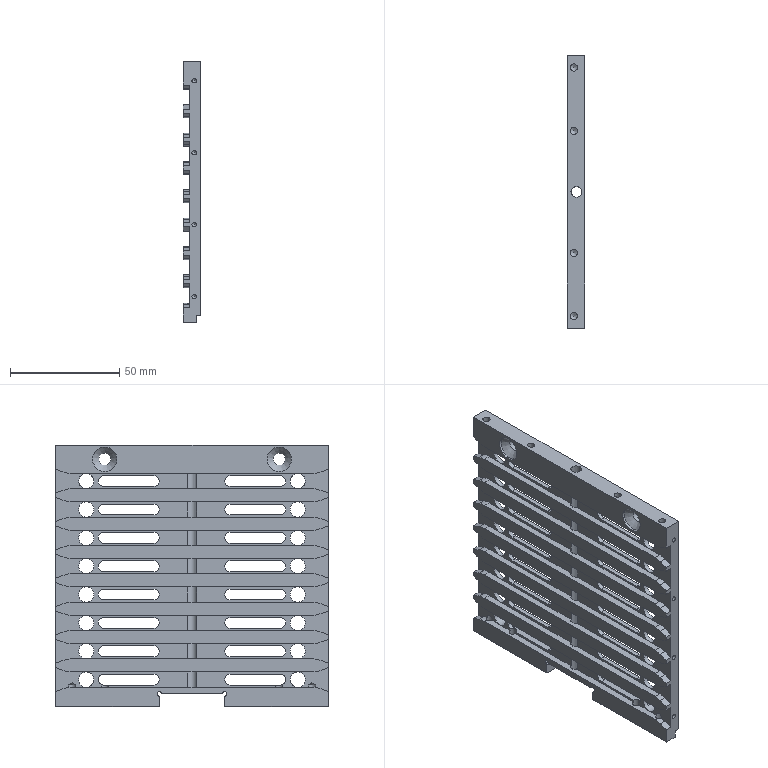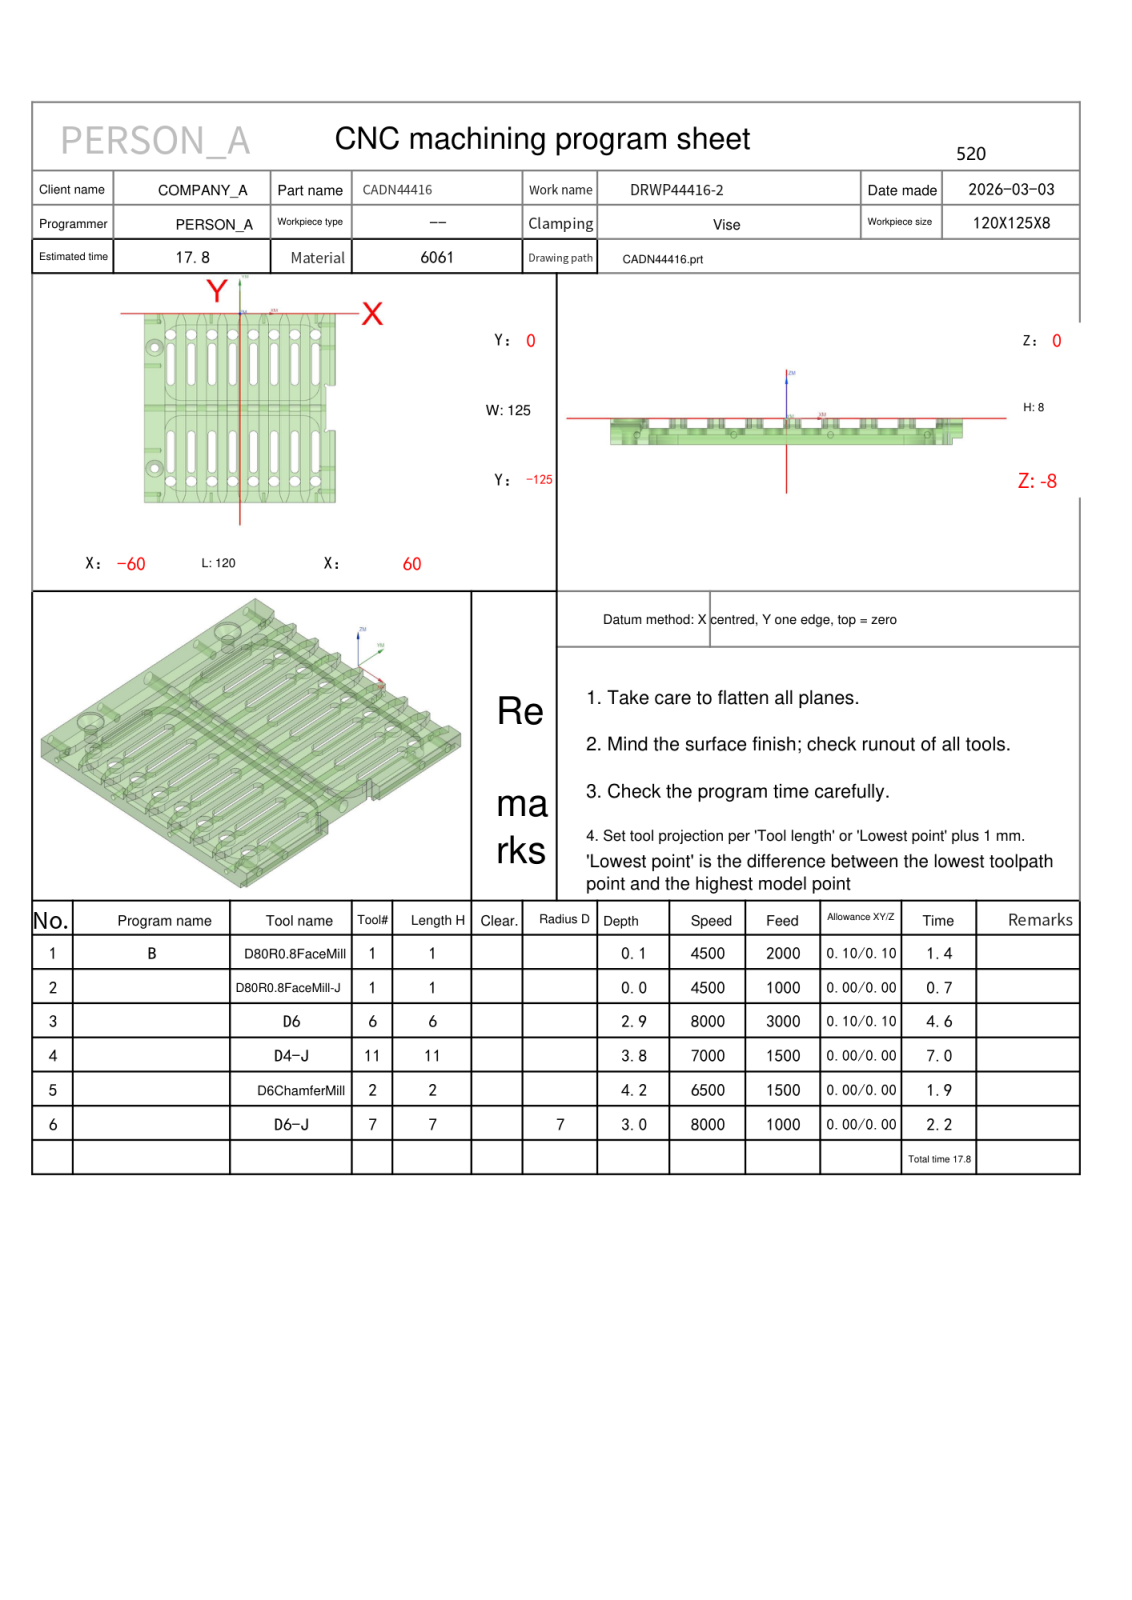NC program | NX | posted by the shop | part box 8 x 125 x 120 mm
Lines 1104 to 2394 of 79132:
N4 T11 M06
(D4-J  D=4. R=0. H=11 ce=0.00 di=0.00)
G00 G90 G54 X-52.886 Y-18.955 M03 S7000
G43 H11 Z50.
M08
Z1.5
G01 X-53.283 Y-18.902 Z1.479 F1500.
X-53.805 Y-18.908 Z1.452
X-54.321 Y-18.99 Z1.424
X-54.82 Y-19.145 Z1.397
X-55.291 Y-19.371 Z1.37
X-55.724 Y-19.663 Z1.342
X-56.111 Y-20.014 Z1.315
X-56.443 Y-20.418 Z1.287
X-56.713 Y-20.865 Z1.26
X-56.915 Y-21.346 Z1.233
X-57.018 Y-21.712 Z1.213
X-57.071 Y-22.009 Z1.197
X-57.1 Y-22.31 Z1.181
Y-22.69 Z1.161
X-57.043 Y-23.164 Z1.136
X-56.925 Y-23.626 Z1.111
X-56.746 Y-24.068 Z1.086
X-56.511 Y-24.483 Z1.061
X-56.222 Y-24.863 Z1.036
X-55.886 Y-25.202 Z1.011
X-55.509 Y-25.494 Z.986
X-55.096 Y-25.733 Z.961
X-54.655 Y-25.915 Z.936
X-54.289 Y-26.018 Z.916
X-53.767 Y-26.095 Z.889
X-53.24 Y-26.096 Z.861
X-52.718 Y-26.019 Z.833
X-52.213 Y-25.867 Z.806
X-51.735 Y-25.643 Z.778
X-51.295 Y-25.352 Z.75
X-50.903 Y-25. Z.723
X-50.566 Y-24.594 Z.695
X-50.291 Y-24.144 Z.667
X-50.086 Y-23.658 Z.64
X-49.983 Y-23.292 Z.62
X-49.905 Y-22.762 Z.592
Y-22.225 Z.564
X-49.986 Y-21.695 Z.536
X-50.144 Y-21.182 Z.507
X-50.377 Y-20.699 Z.479
X-50.679 Y-20.255 Z.451
X-51.043 Y-19.862 Z.423
X-51.462 Y-19.526 Z.395
X-51.786 Y-19.328 Z.375
X-52.263 Y-19.114 Z.348
X-52.765 Y-18.971 Z.32
X-53.283 Y-18.902 Z.293
X-53.805 Y-18.908 Z.266
X-54.321 Y-18.99 Z.238
X-54.82 Y-19.145 Z.211
X-55.291 Y-19.371 Z.183
X-55.724 Y-19.663 Z.156
X-56.111 Y-20.014 Z.129
X-56.443 Y-20.418 Z.101
X-56.713 Y-20.865 Z.074
X-56.915 Y-21.346 Z.047
X-57.018 Y-21.712 Z.027
X-57.071 Y-22.009 Z.011
X-57.1 Y-22.31 Z-.005
Y-22.5 Z-.015
G03 X-53.5 Y-26.1 I3.6 J0.0
X-49.9 Y-22.5 I0.0 J3.6
X-53.5 Y-18.9 I-3.6 J0.0
X-57.1 Y-22.5 I0.0 J-3.6
G01 X-57.091 Y-22.679
X-57.078 Y-22.858
X-57.056 Y-23.036
X-57.024 Y-23.213
X-57.005 Y-23.301 Z-.016
X-56.989 Y-23.389
X-56.961 Y-23.474
X-56.935 Y-23.56
X-56.909 Y-23.646
X-56.879 Y-23.731
X-56.846 Y-23.814
X-56.813 Y-23.898
X-56.739 Y-24.061
X-56.661 Y-24.223
X-56.567 Y-24.376
X-56.471 Y-24.527
X-56.365 Y-24.672 Z-.017
X-56.253 Y-24.813
X-56.194 Y-24.88
X-56.138 Y-24.95
X-56.073 Y-25.012
X-56.009 Y-25.075
X-55.945 Y-25.138
X-55.878 Y-25.198
X-55.809 Y-25.255
X-55.74 Y-25.313
X-55.597 Y-25.421
X-55.451 Y-25.525
X-55.295 Y-25.615 Z-.018
X-55.14 Y-25.705
X-54.976 Y-25.779
X-54.811 Y-25.848
X-54.727 Y-25.879
X-54.644 Y-25.914
X-54.557 Y-25.938
X-54.471 Y-25.962
X-54.38 Y-25.987
X-54.289 Y-26.009
X-54.196 Y-26.027
X-54.104 Y-26.045
X-53.917 Y-26.071
X-53.73 Y-26.093 Z-.019
X-53.542 Y-26.095
X-53.354 Y-26.093
X-53.26 Y-26.087
X-53.166 Y-26.081
X-53.073 Y-26.071
X-52.98 Y-26.057
X-52.886 Y-26.043
X-52.793 Y-26.03
X-52.702 Y-26.006
X-52.611 Y-25.984
X-52.43 Y-25.932
X-52.25 Y-25.876 Z-.02
X-52.077 Y-25.802
X-51.906 Y-25.723
X-51.823 Y-25.68
X-51.739 Y-25.636
X-51.658 Y-25.589
X-51.578 Y-25.539
X-51.499 Y-25.488
X-51.419 Y-25.438
X-51.346 Y-25.379
X-51.271 Y-25.322
X-51.127 Y-25.201
X-50.986 Y-25.076 Z-.021
X-50.858 Y-24.938
X-50.733 Y-24.797
X-50.675 Y-24.723
X-50.616 Y-24.65
X-50.561 Y-24.573
X-50.509 Y-24.495
X-50.457 Y-24.416
X-50.405 Y-24.338
X-50.362 Y-24.254
X-50.316 Y-24.172
X-50.234 Y-24.003
X-50.155 Y-23.832 Z-.022
X-50.095 Y-23.653
X-50.038 Y-23.474
X-50.016 Y-23.387
X-49.994 Y-23.3
X-49.974 Y-23.213
X-49.959 Y-23.124
X-49.944 Y-23.036
X-49.928 Y-22.947
X-49.922 Y-22.858
X-49.915 Y-22.768
X-49.905 Y-22.589
Y-22.41 Z-.023
X-49.915 Y-22.231
X-49.928 Y-22.052
X-49.959 Y-21.875
X-49.994 Y-21.699
X-50.038 Y-21.525
X-50.092 Y-21.354
X-50.122 Y-21.27
X-50.149 Y-21.184
X-50.187 Y-21.103
X-50.223 Y-21.021 Z-.024
X-50.26 Y-20.939
X-50.3 Y-20.858
X-50.343 Y-20.78
X-50.386 Y-20.701
X-50.48 Y-20.548
X-50.578 Y-20.398
X-50.69 Y-20.258
X-50.804 Y-20.119
X-50.927 Y-19.988
X-51.055 Y-19.863
X-51.122 Y-19.803 Z-.025
X-51.187 Y-19.741
X-51.259 Y-19.688
X-51.33 Y-19.633
X-51.402 Y-19.579
X-51.475 Y-19.527
X-51.551 Y-19.479
X-51.626 Y-19.431
X-51.786 Y-19.339
X-51.949 Y-19.251
X-52.119 Y-19.181
X-52.29 Y-19.113
X-52.466 Y-19.056 Z-.026
X-52.644 Y-19.008
X-52.734 Y-18.987
X-52.823 Y-18.964
X-52.914 Y-18.952
X-53.006 Y-18.939
X-53.051 Y-18.932
X-53.097 Y-18.923
X-53.143 Y-18.918
X-53.189 Y-18.917
X-53.281 Y-18.912
X-53.373 Y-18.906
X-53.557 Y-18.905
X-53.742 Y-18.908
X-53.925 Y-18.93 Z-.027
X-54.107 Y-18.956
X-54.198 Y-18.973
X-54.288 Y-18.99
X-54.378 Y-19.013
X-54.467 Y-19.037
X-54.556 Y-19.062
X-54.644 Y-19.09
X-54.73 Y-19.122
X-54.816 Y-19.154
X-54.986 Y-19.226
X-55.154 Y-19.302
X-55.313 Y-19.395 Z-.028
X-55.471 Y-19.492
X-55.546 Y-19.544
X-55.622 Y-19.597
X-55.661 Y-19.621
X-55.698 Y-19.649
X-55.732 Y-19.68
X-55.767 Y-19.71
X-55.839 Y-19.769
X-55.911 Y-19.826
X-55.975 Y-19.892
X-56.041 Y-19.957
X-56.169 Y-20.09
X-56.289 Y-20.229
X-56.401 Y-20.376
X-56.51 Y-20.525 Z-.029
X-56.603 Y-20.684
X-56.692 Y-20.845
X-56.733 Y-20.928
X-56.777 Y-21.009
X-56.81 Y-21.095
X-56.844 Y-21.181
X-56.879 Y-21.267
X-56.909 Y-21.354
X-56.936 Y-21.442
X-56.963 Y-21.53
X-57.003 Y-21.689
X-57.037 Y-21.849 Z-.03
X-57.062 Y-22.011
X-57.085 Y-22.173
X-57.091 Y-22.336
X-57.1 Y-22.5
X-57.091 Y-22.679
X-57.078 Y-22.858
X-57.056 Y-23.036
X-57.024 Y-23.213
X-57.005 Y-23.301 Z-.031
X-56.989 Y-23.389
X-56.961 Y-23.474
X-56.935 Y-23.56
X-56.909 Y-23.646
X-56.879 Y-23.731
X-56.846 Y-23.814
X-56.813 Y-23.898
X-56.739 Y-24.061
X-56.661 Y-24.223
X-56.567 Y-24.376
X-56.471 Y-24.527
X-56.365 Y-24.672 Z-.032
X-56.253 Y-24.812
X-56.194 Y-24.88
X-56.138 Y-24.95
X-56.073 Y-25.012
X-56.009 Y-25.075
X-55.945 Y-25.138
X-55.878 Y-25.198
X-55.809 Y-25.255
X-55.74 Y-25.313
X-55.597 Y-25.421
X-55.451 Y-25.525
X-55.295 Y-25.615 Z-.033
X-55.14 Y-25.705
X-54.976 Y-25.779
X-54.811 Y-25.848
X-54.727 Y-25.879
X-54.644 Y-25.914
X-54.557 Y-25.938
X-54.471 Y-25.962
X-54.38 Y-25.987
X-54.289 Y-26.009
X-54.196 Y-26.027
X-54.104 Y-26.045
X-53.917 Y-26.071
X-53.73 Y-26.093 Z-.034
X-53.542 Y-26.095
X-53.354 Y-26.093
X-53.26 Y-26.087
X-53.166 Y-26.081
X-53.073 Y-26.071
X-52.98 Y-26.057
X-52.886 Y-26.043
X-52.793 Y-26.03
X-52.702 Y-26.006
X-52.611 Y-25.984
X-52.43 Y-25.933
X-52.25 Y-25.876 Z-.035
X-52.077 Y-25.802
X-51.906 Y-25.723
X-51.823 Y-25.68
X-51.739 Y-25.636
X-51.658 Y-25.589
X-51.578 Y-25.539
X-51.499 Y-25.488
X-51.419 Y-25.438
X-51.346 Y-25.379
X-51.271 Y-25.322
X-51.127 Y-25.201
X-50.986 Y-25.076 Z-.036
X-50.858 Y-24.938
X-50.733 Y-24.797
X-50.675 Y-24.723
X-50.616 Y-24.65
X-50.561 Y-24.573
X-50.509 Y-24.495
X-50.457 Y-24.416
X-50.405 Y-24.338
X-50.362 Y-24.254
X-50.316 Y-24.172
X-50.234 Y-24.003
X-50.155 Y-23.832 Z-.037
X-50.095 Y-23.653
X-50.038 Y-23.474
X-50.016 Y-23.387
X-49.994 Y-23.3
X-49.974 Y-23.213
X-49.959 Y-23.124
X-49.944 Y-23.036
X-49.928 Y-22.947
X-49.922 Y-22.858
X-49.915 Y-22.768
X-49.905 Y-22.589
Y-22.41 Z-.038
X-49.915 Y-22.231
X-49.928 Y-22.052
X-49.959 Y-21.875
X-49.994 Y-21.699
X-50.038 Y-21.525
X-50.092 Y-21.354
X-50.122 Y-21.27
X-50.149 Y-21.184
X-50.187 Y-21.103
X-50.223 Y-21.021 Z-.039
X-50.26 Y-20.939
X-50.3 Y-20.858
X-50.343 Y-20.78
X-50.386 Y-20.701
X-50.48 Y-20.548
X-50.578 Y-20.398
X-50.69 Y-20.258
X-50.804 Y-20.119
X-50.927 Y-19.988
X-51.055 Y-19.863
X-51.122 Y-19.803 Z-.04
X-51.187 Y-19.741
X-51.259 Y-19.688
X-51.33 Y-19.633
X-51.402 Y-19.579
X-51.475 Y-19.527
X-51.551 Y-19.479
X-51.626 Y-19.431
X-51.786 Y-19.339
X-51.949 Y-19.251
X-52.119 Y-19.181
X-52.29 Y-19.113
X-52.466 Y-19.056 Z-.041
X-52.644 Y-19.008
X-52.734 Y-18.987
X-52.823 Y-18.964
X-52.914 Y-18.952
X-53.006 Y-18.939
X-53.051 Y-18.932
X-53.097 Y-18.923
X-53.143 Y-18.918
X-53.189 Y-18.917
X-53.281 Y-18.912
X-53.373 Y-18.906
X-53.557 Y-18.905
X-53.742 Y-18.908
X-53.925 Y-18.93 Z-.042
X-54.107 Y-18.956
X-54.198 Y-18.973
X-54.288 Y-18.99
X-54.378 Y-19.013
X-54.467 Y-19.037
X-54.556 Y-19.062
X-54.644 Y-19.09
X-54.73 Y-19.122
X-54.816 Y-19.154
X-54.986 Y-19.226
X-55.154 Y-19.302
X-55.313 Y-19.395 Z-.043
X-55.471 Y-19.492
X-55.546 Y-19.544
X-55.622 Y-19.597
X-55.661 Y-19.621
X-55.698 Y-19.649
X-55.732 Y-19.68
X-55.767 Y-19.71
X-55.839 Y-19.769
X-55.911 Y-19.826
X-55.975 Y-19.892
X-56.041 Y-19.957
X-56.169 Y-20.09
X-56.289 Y-20.229
X-56.401 Y-20.376
X-56.51 Y-20.525 Z-.044
X-56.603 Y-20.684
X-56.692 Y-20.845
X-56.733 Y-20.928
X-56.777 Y-21.009
X-56.81 Y-21.095
X-56.844 Y-21.181
X-56.879 Y-21.267
X-56.909 Y-21.354
X-56.936 Y-21.442
X-56.963 Y-21.53
X-57.003 Y-21.689
X-57.037 Y-21.849 Z-.045
X-57.062 Y-22.011
X-57.085 Y-22.173
X-57.091 Y-22.336
X-57.1 Y-22.5
X-57.091 Y-22.679
X-57.078 Y-22.858
X-57.056 Y-23.036
X-57.024 Y-23.213
X-57.005 Y-23.301 Z-.046
X-56.989 Y-23.389
X-56.961 Y-23.474
X-56.935 Y-23.56
X-56.909 Y-23.646
X-56.879 Y-23.731
X-56.846 Y-23.814
X-56.813 Y-23.898
X-56.739 Y-24.061
X-56.661 Y-24.223
X-56.567 Y-24.376
X-56.471 Y-24.527
X-56.365 Y-24.672 Z-.047
X-56.253 Y-24.812
X-56.194 Y-24.88
X-56.138 Y-24.95
X-56.073 Y-25.012
X-56.009 Y-25.075
X-55.945 Y-25.138
X-55.878 Y-25.198
X-55.809 Y-25.255
X-55.74 Y-25.313
X-55.597 Y-25.421
X-55.451 Y-25.525
X-55.295 Y-25.615 Z-.048
X-55.14 Y-25.705
X-54.976 Y-25.779
X-54.811 Y-25.848
X-54.727 Y-25.879
X-54.644 Y-25.914
X-54.557 Y-25.938
X-54.471 Y-25.962
X-54.38 Y-25.987
X-54.289 Y-26.009
X-54.196 Y-26.027
X-54.104 Y-26.045
X-53.917 Y-26.071
X-53.73 Y-26.093 Z-.049
X-53.542 Y-26.095
X-53.354 Y-26.093
X-53.26 Y-26.087
X-53.166 Y-26.081
X-53.073 Y-26.071
X-52.98 Y-26.057
X-52.886 Y-26.043
X-52.793 Y-26.03
X-52.702 Y-26.006
X-52.611 Y-25.984
X-52.43 Y-25.933
X-52.25 Y-25.876 Z-.05
X-52.077 Y-25.802
X-51.906 Y-25.723
X-51.822 Y-25.68
X-51.739 Y-25.636
X-51.658 Y-25.589
X-51.578 Y-25.539
X-51.499 Y-25.488
X-51.419 Y-25.438
X-51.346 Y-25.379
X-51.271 Y-25.322
X-51.127 Y-25.201
X-50.986 Y-25.076 Z-.051
X-50.858 Y-24.938
X-50.733 Y-24.797
X-50.675 Y-24.723
X-50.616 Y-24.65
X-50.561 Y-24.573
X-50.509 Y-24.495
X-50.457 Y-24.416
X-50.405 Y-24.338
X-50.362 Y-24.254
X-50.316 Y-24.172
X-50.234 Y-24.003
X-50.155 Y-23.832 Z-.052
X-50.095 Y-23.653
X-50.038 Y-23.474
X-50.016 Y-23.387
X-49.994 Y-23.3
X-49.974 Y-23.213
X-49.959 Y-23.124
X-49.944 Y-23.036
X-49.928 Y-22.947
X-49.922 Y-22.858
X-49.915 Y-22.768
X-49.905 Y-22.589
Y-22.41 Z-.053
X-49.915 Y-22.231
X-49.928 Y-22.052
X-49.959 Y-21.875
X-49.994 Y-21.699
X-50.038 Y-21.525
X-50.092 Y-21.354
X-50.122 Y-21.27
X-50.149 Y-21.184
X-50.187 Y-21.103
X-50.223 Y-21.021 Z-.054
X-50.26 Y-20.939
X-50.3 Y-20.858
X-50.343 Y-20.78
X-50.386 Y-20.701
X-50.48 Y-20.548
X-50.578 Y-20.398
X-50.69 Y-20.258
X-50.804 Y-20.119
X-50.927 Y-19.988
X-51.055 Y-19.863
X-51.122 Y-19.803 Z-.055
X-51.187 Y-19.741
X-51.259 Y-19.688
X-51.33 Y-19.633
X-51.402 Y-19.579
X-51.475 Y-19.527
X-51.551 Y-19.479
X-51.626 Y-19.431
X-51.786 Y-19.339
X-51.949 Y-19.251
X-52.119 Y-19.181
X-52.29 Y-19.113
X-52.466 Y-19.056 Z-.056
X-52.644 Y-19.008
X-52.734 Y-18.987
X-52.823 Y-18.964
X-52.914 Y-18.952
X-53.006 Y-18.939
X-53.051 Y-18.932
X-53.097 Y-18.923
X-53.143 Y-18.918
X-53.189 Y-18.917
X-53.281 Y-18.912
X-53.373 Y-18.906
X-53.557 Y-18.905
X-53.742 Y-18.908
X-53.925 Y-18.93 Z-.057
X-54.107 Y-18.956
X-54.198 Y-18.973
X-54.288 Y-18.99
X-54.378 Y-19.013
X-54.467 Y-19.037
X-54.556 Y-19.062
X-54.644 Y-19.09
X-54.73 Y-19.122
X-54.816 Y-19.154
X-54.986 Y-19.226
X-55.154 Y-19.302
X-55.313 Y-19.396 Z-.058
X-55.471 Y-19.492
X-55.546 Y-19.544
X-55.622 Y-19.597
X-55.661 Y-19.621
X-55.698 Y-19.649
X-55.732 Y-19.68
X-55.767 Y-19.71
X-55.838 Y-19.769
X-55.911 Y-19.826
X-55.975 Y-19.892
X-56.041 Y-19.957
X-56.169 Y-20.09
X-56.289 Y-20.229
X-56.401 Y-20.376
X-56.51 Y-20.525 Z-.059
X-56.603 Y-20.684
X-56.692 Y-20.845
X-56.733 Y-20.928
X-56.777 Y-21.009
X-56.81 Y-21.095
X-56.844 Y-21.181
X-56.879 Y-21.267
X-56.909 Y-21.354
X-56.936 Y-21.442
X-56.963 Y-21.53
X-57.003 Y-21.689
X-57.037 Y-21.849 Z-.06
X-57.062 Y-22.011
X-57.085 Y-22.173
X-57.091 Y-22.336
X-57.1 Y-22.5
X-57.091 Y-22.679
X-57.078 Y-22.858
X-57.056 Y-23.036
X-57.024 Y-23.213
X-57.005 Y-23.301 Z-.061
X-56.989 Y-23.389
X-56.961 Y-23.474
X-56.935 Y-23.56
X-56.909 Y-23.646
X-56.879 Y-23.731
X-56.846 Y-23.814
X-56.813 Y-23.898
X-56.739 Y-24.061
X-56.661 Y-24.223
X-56.567 Y-24.376
X-56.471 Y-24.527
X-56.365 Y-24.672 Z-.062
X-56.253 Y-24.812
X-56.194 Y-24.88
X-56.138 Y-24.95
X-56.073 Y-25.012
X-56.009 Y-25.075
X-55.945 Y-25.138
X-55.878 Y-25.198
X-55.809 Y-25.255
X-55.74 Y-25.313
X-55.597 Y-25.421
X-55.451 Y-25.525
X-55.295 Y-25.615 Z-.063
X-55.14 Y-25.705
X-54.976 Y-25.779
X-54.811 Y-25.848
X-54.727 Y-25.879
X-54.644 Y-25.914
X-54.557 Y-25.938
X-54.471 Y-25.962
X-54.38 Y-25.987
X-54.289 Y-26.009
X-54.196 Y-26.027
X-54.104 Y-26.045
X-53.917 Y-26.071
X-53.73 Y-26.093 Z-.064
X-53.542 Y-26.095
X-53.354 Y-26.093
X-53.26 Y-26.087
X-53.166 Y-26.081
X-53.073 Y-26.071
X-52.98 Y-26.057
X-52.886 Y-26.043
X-52.793 Y-26.03
X-52.702 Y-26.006
X-52.611 Y-25.984
X-52.43 Y-25.933
X-52.25 Y-25.876 Z-.065
X-52.077 Y-25.802
X-51.906 Y-25.723
X-51.822 Y-25.68
X-51.739 Y-25.636
X-51.658 Y-25.589
X-51.578 Y-25.539
X-51.499 Y-25.488
X-51.419 Y-25.438
X-51.346 Y-25.379
X-51.271 Y-25.322
X-51.127 Y-25.201
X-50.986 Y-25.076 Z-.066
X-50.858 Y-24.938
X-50.733 Y-24.797
X-50.675 Y-24.723
X-50.616 Y-24.65
X-50.561 Y-24.573
X-50.509 Y-24.495
X-50.457 Y-24.416
X-50.405 Y-24.338
X-50.362 Y-24.254
X-50.316 Y-24.172
X-50.234 Y-24.003
X-50.155 Y-23.832 Z-.067
X-50.095 Y-23.653
X-50.038 Y-23.474
X-50.016 Y-23.387
X-49.994 Y-23.3
X-49.974 Y-23.213
X-49.959 Y-23.124
X-49.944 Y-23.036
X-49.928 Y-22.947
X-49.922 Y-22.858
X-49.915 Y-22.768
X-49.905 Y-22.589
Y-22.41 Z-.068
X-49.915 Y-22.231
X-49.928 Y-22.052
X-49.959 Y-21.875
X-49.994 Y-21.699
X-50.038 Y-21.525
X-50.092 Y-21.354
X-50.121 Y-21.269
X-50.149 Y-21.184
X-50.187 Y-21.103
X-50.223 Y-21.021 Z-.069
X-50.26 Y-20.939
X-50.3 Y-20.858
X-50.343 Y-20.78
X-50.386 Y-20.701
X-50.48 Y-20.548
X-50.578 Y-20.398
X-50.69 Y-20.258
X-50.804 Y-20.119
X-50.927 Y-19.988
X-51.055 Y-19.863
X-51.122 Y-19.803 Z-.07
X-51.187 Y-19.741
X-51.259 Y-19.688
X-51.33 Y-19.633
X-51.402 Y-19.579
X-51.475 Y-19.527
X-51.551 Y-19.479
X-51.626 Y-19.431
X-51.786 Y-19.339
X-51.949 Y-19.251
X-52.119 Y-19.181
X-52.29 Y-19.113
X-52.466 Y-19.056 Z-.071
X-52.644 Y-19.008
X-52.734 Y-18.987
X-52.823 Y-18.964
X-52.914 Y-18.952
X-53.006 Y-18.939
X-53.051 Y-18.932
X-53.097 Y-18.923
X-53.143 Y-18.918
X-53.189 Y-18.917
X-53.281 Y-18.912
X-53.373 Y-18.906
X-53.557 Y-18.905
X-53.742 Y-18.908
X-53.925 Y-18.93 Z-.072
X-54.107 Y-18.956
X-54.198 Y-18.973
X-54.288 Y-18.99
X-54.378 Y-19.013
X-54.467 Y-19.037
X-54.556 Y-19.062
X-54.644 Y-19.09
X-54.73 Y-19.122
X-54.816 Y-19.154
X-54.986 Y-19.226
X-55.154 Y-19.302
X-55.313 Y-19.396 Z-.073
X-55.471 Y-19.492
X-55.546 Y-19.544
X-55.622 Y-19.597
X-55.661 Y-19.621
X-55.698 Y-19.649
X-55.732 Y-19.68
X-55.767 Y-19.71
X-55.838 Y-19.769
X-55.911 Y-19.826
X-55.975 Y-19.892
X-56.041 Y-19.957
X-56.169 Y-20.09
X-56.289 Y-20.229
X-56.401 Y-20.376
X-56.51 Y-20.525 Z-.074
X-56.603 Y-20.684
X-56.692 Y-20.845
X-56.733 Y-20.928
X-56.777 Y-21.009
X-56.81 Y-21.095
X-56.844 Y-21.181
X-56.879 Y-21.267
X-56.909 Y-21.354
X-56.936 Y-21.442
X-56.963 Y-21.53
X-57.003 Y-21.689
X-57.037 Y-21.849 Z-.075
X-57.062 Y-22.011
X-57.085 Y-22.173
X-57.091 Y-22.336
X-57.1 Y-22.5
X-57.091 Y-22.679
X-57.078 Y-22.858
X-57.056 Y-23.036
X-57.024 Y-23.213
X-57.005 Y-23.301 Z-.076
X-56.989 Y-23.389
X-56.961 Y-23.474
X-56.935 Y-23.56
X-56.909 Y-23.646
X-56.879 Y-23.731
X-56.846 Y-23.814
X-56.813 Y-23.898
X-56.739 Y-24.061
X-56.661 Y-24.223
X-56.567 Y-24.376
X-56.471 Y-24.527
X-56.365 Y-24.672 Z-.077
X-56.253 Y-24.812
X-56.194 Y-24.88
X-56.138 Y-24.95
X-56.073 Y-25.012
X-56.009 Y-25.075
X-55.945 Y-25.138
X-55.878 Y-25.198
X-55.809 Y-25.255
X-55.74 Y-25.313
X-55.597 Y-25.421
X-55.451 Y-25.525
X-55.295 Y-25.615 Z-.078
X-55.14 Y-25.705
X-54.976 Y-25.779
X-54.811 Y-25.848
X-54.727 Y-25.879
X-54.644 Y-25.914
X-54.557 Y-25.938
X-54.471 Y-25.962
X-54.38 Y-25.987
X-54.289 Y-26.009
X-54.196 Y-26.027
X-54.104 Y-26.045
X-53.917 Y-26.071
X-53.73 Y-26.093 Z-.079
X-53.542 Y-26.095
X-53.354 Y-26.093
X-53.26 Y-26.087
X-53.166 Y-26.081
X-53.073 Y-26.071
X-52.98 Y-26.057
X-52.886 Y-26.043
X-52.793 Y-26.03
X-52.702 Y-26.006
X-52.611 Y-25.984
X-52.43 Y-25.933
X-52.25 Y-25.876 Z-.08
X-52.077 Y-25.802
X-51.906 Y-25.723
X-51.822 Y-25.68
X-51.739 Y-25.636
X-51.658 Y-25.589
X-51.578 Y-25.539
X-51.499 Y-25.488
X-51.419 Y-25.438
X-51.346 Y-25.379
X-51.271 Y-25.322
X-51.127 Y-25.201
X-50.986 Y-25.076 Z-.081
X-50.858 Y-24.938
X-50.733 Y-24.797
X-50.675 Y-24.723
X-50.616 Y-24.65
X-50.561 Y-24.573
X-50.509 Y-24.495
X-50.457 Y-24.416
X-50.405 Y-24.338
X-50.362 Y-24.254
X-50.316 Y-24.172
X-50.234 Y-24.003
X-50.155 Y-23.832 Z-.082
X-50.095 Y-23.653
X-50.038 Y-23.474
X-50.016 Y-23.387
X-49.994 Y-23.3
X-49.974 Y-23.213
X-49.959 Y-23.124
X-49.944 Y-23.036
X-49.928 Y-22.947
X-49.922 Y-22.858
X-49.915 Y-22.768
X-49.905 Y-22.589
Y-22.41 Z-.083
X-49.915 Y-22.231
X-49.928 Y-22.052
X-49.959 Y-21.875
X-49.994 Y-21.699
X-50.038 Y-21.525
X-50.092 Y-21.354
X-50.121 Y-21.269
X-50.149 Y-21.184
X-50.187 Y-21.103
X-50.223 Y-21.021 Z-.084
X-50.26 Y-20.939
X-50.3 Y-20.858
X-50.343 Y-20.78
X-50.386 Y-20.701
X-50.48 Y-20.548
X-50.578 Y-20.398
X-50.69 Y-20.258
X-50.804 Y-20.119
X-50.927 Y-19.988
X-51.055 Y-19.863
X-51.122 Y-19.803 Z-.085
X-51.187 Y-19.741
X-51.259 Y-19.688
X-51.33 Y-19.633
X-51.402 Y-19.579
X-51.475 Y-19.527
X-51.551 Y-19.479
X-51.626 Y-19.431
X-51.786 Y-19.339
X-51.949 Y-19.251
X-52.119 Y-19.181
X-52.29 Y-19.113
X-52.466 Y-19.056 Z-.086
X-52.644 Y-19.008
X-52.734 Y-18.987
X-52.823 Y-18.964
X-52.914 Y-18.952
X-53.006 Y-18.939
X-53.051 Y-18.932
X-53.097 Y-18.923
X-53.143 Y-18.918
X-53.189 Y-18.917
X-53.281 Y-18.912
X-53.373 Y-18.906
X-53.557 Y-18.905
X-53.742 Y-18.908
X-53.925 Y-18.93 Z-.087
X-54.107 Y-18.956
X-54.198 Y-18.973
X-54.288 Y-18.99
X-54.378 Y-19.013
X-54.467 Y-19.037
X-54.556 Y-19.062
X-54.644 Y-19.09
X-54.73 Y-19.122
X-54.816 Y-19.154
X-54.986 Y-19.226
X-55.154 Y-19.302
X-55.313 Y-19.396 Z-.088
X-55.471 Y-19.492
X-55.546 Y-19.544
X-55.622 Y-19.597
X-55.661 Y-19.621
X-55.698 Y-19.649
X-55.732 Y-19.68
X-55.767 Y-19.71
X-55.838 Y-19.769
X-55.911 Y-19.826
X-55.975 Y-19.892
X-56.041 Y-19.957
X-56.169 Y-20.09
X-56.289 Y-20.229
X-56.401 Y-20.376
X-56.51 Y-20.525 Z-.089
X-56.603 Y-20.684
X-56.692 Y-20.845
X-56.733 Y-20.928
X-56.777 Y-21.009
X-56.81 Y-21.095
X-56.844 Y-21.181
X-56.879 Y-21.267
X-56.909 Y-21.354
X-56.936 Y-21.442
X-56.963 Y-21.53
X-57.003 Y-21.689
X-57.037 Y-21.849 Z-.09
X-57.062 Y-22.011
X-57.085 Y-22.173
X-57.091 Y-22.336
X-57.1 Y-22.5
X-57.091 Y-22.679
X-57.078 Y-22.858
X-57.056 Y-23.036
X-57.024 Y-23.213
X-57.005 Y-23.301 Z-.091
X-56.989 Y-23.389
X-56.961 Y-23.474
X-56.935 Y-23.56
X-56.909 Y-23.646
X-56.879 Y-23.731
X-56.846 Y-23.814
X-56.813 Y-23.898
X-56.739 Y-24.061
X-56.661 Y-24.223
X-56.567 Y-24.376
X-56.471 Y-24.527
X-56.365 Y-24.672 Z-.092
X-56.253 Y-24.812
X-56.194 Y-24.88
X-56.138 Y-24.95
X-56.073 Y-25.012
X-56.009 Y-25.075
X-55.945 Y-25.138
X-55.878 Y-25.198
X-55.809 Y-25.255
X-55.74 Y-25.313
X-55.597 Y-25.421
X-55.451 Y-25.525
X-55.295 Y-25.615 Z-.093
X-55.14 Y-25.705
X-54.976 Y-25.779
X-54.811 Y-25.848
X-54.727 Y-25.879
X-54.644 Y-25.914
X-54.557 Y-25.938
X-54.471 Y-25.962
X-54.38 Y-25.987
X-54.289 Y-26.009
X-54.196 Y-26.027
X-54.104 Y-26.045
X-53.917 Y-26.071
X-53.73 Y-26.093 Z-.094
X-53.542 Y-26.095
X-53.354 Y-26.093
X-53.26 Y-26.087
X-53.166 Y-26.081
X-53.073 Y-26.071
X-52.98 Y-26.057
X-52.886 Y-26.043
X-52.793 Y-26.03
X-52.702 Y-26.006
X-52.611 Y-25.984
X-52.43 Y-25.933
X-52.25 Y-25.876 Z-.095
X-52.077 Y-25.802
X-51.906 Y-25.723
X-51.822 Y-25.68
X-51.739 Y-25.636
X-51.658 Y-25.589
X-51.578 Y-25.539
X-51.499 Y-25.488
X-51.419 Y-25.438
X-51.346 Y-25.379
X-51.271 Y-25.322
X-51.127 Y-25.201
X-50.986 Y-25.076 Z-.096
X-50.858 Y-24.938
X-50.733 Y-24.797
X-50.675 Y-24.723
X-50.616 Y-24.65
X-50.561 Y-24.573
X-50.509 Y-24.495
X-50.457 Y-24.416
X-50.405 Y-24.338
X-50.362 Y-24.254
X-50.316 Y-24.172
X-50.234 Y-24.003
X-50.155 Y-23.832 Z-.097
X-50.095 Y-23.653
X-50.038 Y-23.474
X-50.016 Y-23.387
X-49.994 Y-23.3
X-49.974 Y-23.213
X-49.959 Y-23.124
X-49.944 Y-23.036
X-49.928 Y-22.947
X-49.922 Y-22.858
X-49.915 Y-22.768
X-49.905 Y-22.589
Y-22.41 Z-.098
X-49.915 Y-22.231
X-49.928 Y-22.052
X-49.959 Y-21.875
X-49.994 Y-21.699
X-50.038 Y-21.525
X-50.092 Y-21.354
X-50.121 Y-21.269
X-50.149 Y-21.184
X-50.187 Y-21.103
X-50.223 Y-21.021 Z-.099
X-50.26 Y-20.939
X-50.3 Y-20.858
X-50.343 Y-20.78
X-50.386 Y-20.701
X-50.48 Y-20.548
X-50.578 Y-20.398
X-50.69 Y-20.258
X-50.804 Y-20.119
X-50.927 Y-19.988
X-51.055 Y-19.863
X-51.122 Y-19.803 Z-.1
X-51.187 Y-19.741
X-51.259 Y-19.688
X-51.33 Y-19.633
X-51.402 Y-19.579
X-51.475 Y-19.527
X-51.551 Y-19.479
X-51.626 Y-19.431
X-51.786 Y-19.339
X-51.949 Y-19.251
X-52.119 Y-19.181
X-52.29 Y-19.113
X-52.466 Y-19.056 Z-.101
X-52.644 Y-19.008
X-52.734 Y-18.987
X-52.823 Y-18.964
X-52.914 Y-18.952
X-53.006 Y-18.939
X-53.051 Y-18.932
X-53.097 Y-18.923
X-53.143 Y-18.918
X-53.189 Y-18.917
X-53.281 Y-18.912
X-53.373 Y-18.906
X-53.557 Y-18.905
X-53.742 Y-18.908
X-53.925 Y-18.93 Z-.102
X-54.107 Y-18.956
X-54.198 Y-18.973
X-54.288 Y-18.99
X-54.378 Y-19.013
X-54.467 Y-19.037
X-54.556 Y-19.062
X-54.644 Y-19.09
X-54.73 Y-19.122
X-54.816 Y-19.154
X-54.986 Y-19.226
X-55.154 Y-19.302
X-55.313 Y-19.396 Z-.103
X-55.471 Y-19.492
X-55.546 Y-19.544
X-55.622 Y-19.597
X-55.661 Y-19.621
X-55.698 Y-19.649
X-55.732 Y-19.68
X-55.767 Y-19.71
X-55.838 Y-19.769
X-55.911 Y-19.826
X-55.975 Y-19.892
X-56.041 Y-19.957
X-56.169 Y-20.09
X-56.289 Y-20.229
X-56.401 Y-20.376
X-56.51 Y-20.525 Z-.104
X-56.603 Y-20.684
X-56.692 Y-20.845
X-56.733 Y-20.928
X-56.777 Y-21.009
X-56.81 Y-21.095
X-56.844 Y-21.181
X-56.878 Y-21.267
X-56.909 Y-21.354
X-56.936 Y-21.442
X-56.963 Y-21.53
X-57.003 Y-21.689
X-57.037 Y-21.849 Z-.105
X-57.062 Y-22.011
X-57.085 Y-22.173
X-57.091 Y-22.336
X-57.1 Y-22.5
X-57.091 Y-22.679
X-57.078 Y-22.858
X-57.056 Y-23.036
X-57.024 Y-23.213
X-57.005 Y-23.301 Z-.106
X-56.989 Y-23.389
X-56.961 Y-23.474
X-56.935 Y-23.56
X-56.909 Y-23.646
X-56.879 Y-23.731
X-56.846 Y-23.814
X-56.813 Y-23.898
X-56.739 Y-24.061
X-56.661 Y-24.223
X-56.567 Y-24.376
X-56.471 Y-24.527
X-56.365 Y-24.672 Z-.107
X-56.253 Y-24.812
X-56.194 Y-24.88
X-56.138 Y-24.95
X-56.073 Y-25.012
X-56.009 Y-25.075
X-55.945 Y-25.138
X-55.878 Y-25.198
X-55.809 Y-25.255
X-55.74 Y-25.313
X-55.597 Y-25.421
X-55.451 Y-25.525
X-55.295 Y-25.615 Z-.108
X-55.14 Y-25.705
X-54.976 Y-25.779
X-54.811 Y-25.848
X-54.727 Y-25.879
X-54.644 Y-25.914
X-54.557 Y-25.938
X-54.471 Y-25.962
X-54.38 Y-25.987
X-54.289 Y-26.009
X-54.196 Y-26.027
X-54.104 Y-26.045
X-53.917 Y-26.071
X-53.73 Y-26.093 Z-.109
X-53.542 Y-26.095
X-53.354 Y-26.093
X-53.26 Y-26.087
X-53.166 Y-26.081
X-53.073 Y-26.071
X-52.98 Y-26.057
X-52.886 Y-26.043
X-52.793 Y-26.03
X-52.702 Y-26.006
X-52.611 Y-25.984
X-52.43 Y-25.933
X-52.25 Y-25.876 Z-.11
X-52.077 Y-25.802
X-51.906 Y-25.723
X-51.823 Y-25.68
X-51.739 Y-25.636
X-51.658 Y-25.589
X-51.578 Y-25.539
X-51.499 Y-25.488
X-51.419 Y-25.438
X-51.346 Y-25.379
X-51.271 Y-25.322
X-51.127 Y-25.201
X-50.986 Y-25.076 Z-.111
X-50.858 Y-24.938
X-50.733 Y-24.797
X-50.675 Y-24.723
X-50.616 Y-24.65
X-50.561 Y-24.573
X-50.509 Y-24.495
X-50.457 Y-24.416
X-50.405 Y-24.338
X-50.362 Y-24.254
X-50.316 Y-24.172
X-50.234 Y-24.003
X-50.155 Y-23.832 Z-.112
X-50.095 Y-23.653
X-50.038 Y-23.474
X-50.016 Y-23.387
X-49.994 Y-23.3
X-49.974 Y-23.213
X-49.959 Y-23.124
X-49.944 Y-23.036
X-49.928 Y-22.947
X-49.922 Y-22.858
X-49.915 Y-22.768
X-49.905 Y-22.589
Y-22.41 Z-.113
X-49.915 Y-22.231
X-49.928 Y-22.052
X-49.959 Y-21.875
X-49.994 Y-21.699
X-50.038 Y-21.525
X-50.092 Y-21.354
X-50.121 Y-21.269
X-50.149 Y-21.184
X-50.187 Y-21.103
X-50.223 Y-21.021 Z-.114
X-50.26 Y-20.939
X-50.3 Y-20.858
X-50.343 Y-20.78
X-50.386 Y-20.701
X-50.48 Y-20.548
X-50.578 Y-20.398
X-50.69 Y-20.258
X-50.804 Y-20.119
X-50.927 Y-19.988
X-51.055 Y-19.863
X-51.122 Y-19.803 Z-.115
X-51.187 Y-19.741
X-51.259 Y-19.688
X-51.33 Y-19.633
X-51.402 Y-19.579
X-51.475 Y-19.527
X-51.551 Y-19.479
X-51.626 Y-19.431
X-51.786 Y-19.339
X-51.949 Y-19.251
X-52.119 Y-19.181
X-52.29 Y-19.113
X-52.466 Y-19.056 Z-.116
X-52.644 Y-19.008
X-52.734 Y-18.987
X-52.823 Y-18.964
X-52.914 Y-18.952
X-53.006 Y-18.939
X-53.051 Y-18.932
X-53.097 Y-18.923
X-53.143 Y-18.918
X-53.189 Y-18.917
X-53.281 Y-18.912
X-53.373 Y-18.906
X-53.557 Y-18.905
X-53.742 Y-18.908
X-53.925 Y-18.93 Z-.117
X-54.107 Y-18.956
X-54.198 Y-18.973
X-54.288 Y-18.99
X-54.378 Y-19.013